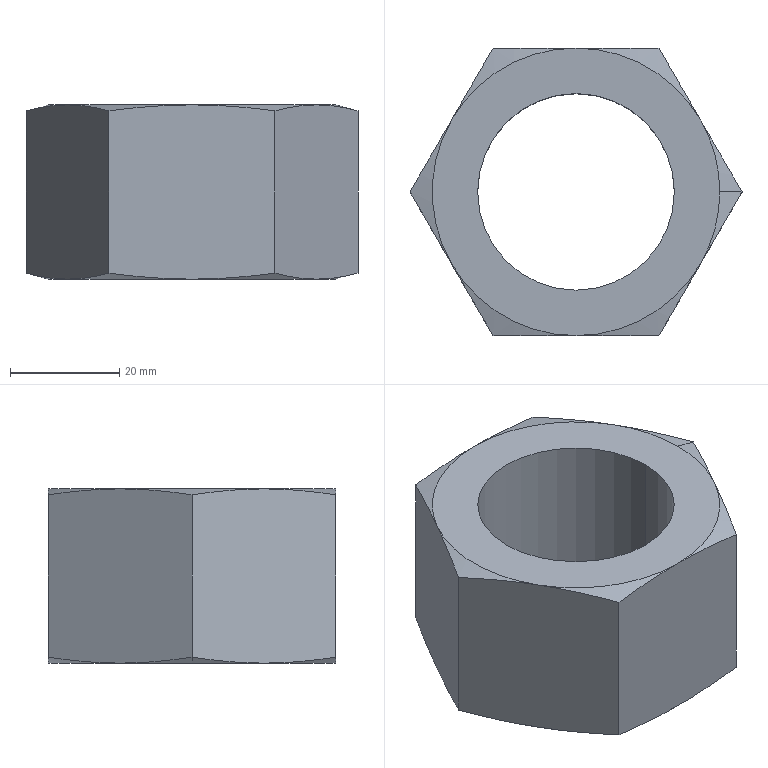Part | SolidWorks | features Cut 2, Chamfer 1, Extrusion 1 | 1 solid | 24 faces | box 60.79 x 52.646 x 31.9 mm | volume 43950 mm3 | cone 14 | plane 8 | cylinder 2 | commonest cylinder face diameters 36 x2
STEP:
#1=CARTESIAN_POINT('',(22.796,13.161,31.9));
#2=VERTEX_POINT('',#1);
#3=CARTESIAN_POINT('',(26.323,0.,31.9));
#4=VERTEX_POINT('',#3);
#5=CARTESIAN_POINT('',(0.,0.,31.9));
#6=DIRECTION('',(0.,0.,-1.));
#7=DIRECTION('',(-1.,0.,0.));
#8=AXIS2_PLACEMENT_3D('',#5,#6,#7);
#9=CIRCLE('',#8,26.323);
#10=EDGE_CURVE('',#2,#4,#9,.T.);
#11=ORIENTED_EDGE('',*,*,#10,.T.);
#12=CARTESIAN_POINT('',(30.395,0.,30.809));
#13=VERTEX_POINT('',#12);
#14=CARTESIAN_POINT('',(26.323,0.,31.9));
#15=DIRECTION('',(0.9659,0.,-0.2588));
#16=VECTOR('',#15,1000.);
#17=LINE('',#14,#16);
#18=EDGE_CURVE('',#4,#13,#17,.T.);
#19=ORIENTED_EDGE('',*,*,#18,.T.);
#20=CARTESIAN_POINT('',(30.395,0.,30.809));
#21=CARTESIAN_POINT('',(29.129,2.194,31.148));
#22=CARTESIAN_POINT('',(27.862,4.387,31.424));
#23=CARTESIAN_POINT('',(25.329,8.774,31.8));
#24=CARTESIAN_POINT('',(24.063,10.968,31.9));
#25=CARTESIAN_POINT('',(22.796,13.161,31.9));
#26=B_SPLINE_CURVE_WITH_KNOTS('',3,(#20,#21,#22,#23,#24,#25),.UNSPECIFIED.,.F.,.F.,(4,2,4),(0.000000231,0.007599,0.0152),.UNSPECIFIED.);
#27=EDGE_CURVE('',#13,#2,#26,.T.);
#28=ORIENTED_EDGE('',*,*,#27,.T.);
#29=EDGE_LOOP('',(#11,#19,#28));
#30=FACE_OUTER_BOUND('',#29,.T.);
#31=CARTESIAN_POINT('',(0.,0.,31.9));
#32=DIRECTION('',(0.,0.,-1.));
#33=DIRECTION('',(1.,0.,0.));
#34=AXIS2_PLACEMENT_3D('',#31,#32,#33);
#35=CONICAL_SURFACE('',#34,26.323,1.309);
#36=ADVANCED_FACE('',(#30),#35,.T.);
#37=CARTESIAN_POINT('',(-26.323,0.,0.));
#38=VERTEX_POINT('',#37);
#39=CARTESIAN_POINT('',(-22.796,13.161,0.));
#40=VERTEX_POINT('',#39);
#41=CARTESIAN_POINT('',(0.,0.,0.));
#42=DIRECTION('',(0.,0.,-1.));
#43=DIRECTION('',(-1.,0.,0.));
#44=AXIS2_PLACEMENT_3D('',#41,#42,#43);
#45=CIRCLE('',#44,26.323);
#46=EDGE_CURVE('',#38,#40,#45,.T.);
#47=ORIENTED_EDGE('',*,*,#46,.F.);
#48=CARTESIAN_POINT('',(-30.395,0.,1.091));
#49=VERTEX_POINT('',#48);
#50=CARTESIAN_POINT('',(-26.323,0.,0.));
#51=DIRECTION('',(-0.9659,0.,0.2588));
#52=VECTOR('',#51,1000.);
#53=LINE('',#50,#52);
#54=EDGE_CURVE('',#38,#49,#53,.T.);
#55=ORIENTED_EDGE('',*,*,#54,.T.);
#56=CARTESIAN_POINT('',(-30.395,0.,1.091));
#57=CARTESIAN_POINT('',(-29.129,2.194,0.7518));
#58=CARTESIAN_POINT('',(-27.862,4.387,0.4762));
#59=CARTESIAN_POINT('',(-25.329,8.774,0.09977));
#60=CARTESIAN_POINT('',(-24.063,10.968,0.));
#61=CARTESIAN_POINT('',(-22.796,13.161,0.));
#62=B_SPLINE_CURVE_WITH_KNOTS('',3,(#56,#57,#58,#59,#60,#61),.UNSPECIFIED.,.F.,.F.,(4,2,4),(0.000000231,0.007599,0.0152),.UNSPECIFIED.);
#63=EDGE_CURVE('',#49,#40,#62,.T.);
#64=ORIENTED_EDGE('',*,*,#63,.T.);
#65=EDGE_LOOP('',(#47,#55,#64));
#66=FACE_OUTER_BOUND('',#65,.T.);
#67=CARTESIAN_POINT('',(0.,0.,0.));
#68=DIRECTION('',(0.,0.,1.));
#69=DIRECTION('',(-1.,0.,0.));
#70=AXIS2_PLACEMENT_3D('',#67,#68,#69);
#71=CONICAL_SURFACE('',#70,26.323,1.309);
#72=ADVANCED_FACE('',(#66),#71,.T.);
#73=CARTESIAN_POINT('',(-18.,0.,31.9));
#74=VERTEX_POINT('',#73);
#75=CARTESIAN_POINT('',(18.,0.,31.9));
#76=VERTEX_POINT('',#75);
#77=CARTESIAN_POINT('',(0.,0.,31.9));
#78=DIRECTION('',(0.,0.,1.));
#79=DIRECTION('',(1.,0.,0.));
#80=AXIS2_PLACEMENT_3D('',#77,#78,#79);
#81=CIRCLE('',#80,18.);
#82=EDGE_CURVE('',#74,#76,#81,.T.);
#83=ORIENTED_EDGE('',*,*,#82,.T.);
#84=CARTESIAN_POINT('',(18.,0.,0.));
#85=VERTEX_POINT('',#84);
#86=CARTESIAN_POINT('',(18.,0.,31.9));
#87=DIRECTION('',(0.,0.,-1.));
#88=VECTOR('',#87,1000.);
#89=LINE('',#86,#88);
#90=EDGE_CURVE('',#76,#85,#89,.T.);
#91=ORIENTED_EDGE('',*,*,#90,.T.);
#92=CARTESIAN_POINT('',(-18.,0.,0.));
#93=VERTEX_POINT('',#92);
#94=CARTESIAN_POINT('',(0.,0.,0.));
#95=DIRECTION('',(0.,0.,1.));
#96=DIRECTION('',(1.,0.,0.));
#97=AXIS2_PLACEMENT_3D('',#94,#95,#96);
#98=CIRCLE('',#97,18.);
#99=EDGE_CURVE('',#93,#85,#98,.T.);
#100=ORIENTED_EDGE('',*,*,#99,.F.);
#101=CARTESIAN_POINT('',(-18.,0.,31.9));
#102=DIRECTION('',(0.,0.,-1.));
#103=VECTOR('',#102,1000.);
#104=LINE('',#101,#103);
#105=EDGE_CURVE('',#74,#93,#104,.T.);
#106=ORIENTED_EDGE('',*,*,#105,.F.);
#107=EDGE_LOOP('',(#83,#91,#100,#106));
#108=FACE_OUTER_BOUND('',#107,.T.);
#109=CARTESIAN_POINT('',(0.,0.,31.9));
#110=DIRECTION('',(0.,0.,-1.));
#111=DIRECTION('',(-1.,0.,0.));
#112=AXIS2_PLACEMENT_3D('',#109,#110,#111);
#113=CYLINDRICAL_SURFACE('',#112,18.);
#114=ADVANCED_FACE('',(#108),#113,.F.);
#115=ORIENTED_EDGE('',*,*,#27,.F.);
#116=CARTESIAN_POINT('',(30.395,0.,1.091));
#117=VERTEX_POINT('',#116);
#118=CARTESIAN_POINT('',(30.395,0.,31.9));
#119=DIRECTION('',(0.,0.,-1.));
#120=VECTOR('',#119,1000.);
#121=LINE('',#118,#120);
#122=EDGE_CURVE('',#13,#117,#121,.T.);
#123=ORIENTED_EDGE('',*,*,#122,.T.);
#124=CARTESIAN_POINT('',(22.796,13.161,0.));
#125=VERTEX_POINT('',#124);
#126=CARTESIAN_POINT('',(22.796,13.161,0.));
#127=CARTESIAN_POINT('',(24.063,10.968,0.));
#128=CARTESIAN_POINT('',(25.329,8.774,0.09977));
#129=CARTESIAN_POINT('',(27.862,4.387,0.4762));
#130=CARTESIAN_POINT('',(29.129,2.194,0.7518));
#131=CARTESIAN_POINT('',(30.395,0.,1.091));
#132=B_SPLINE_CURVE_WITH_KNOTS('',3,(#126,#127,#128,#129,#130,#131),.UNSPECIFIED.,.F.,.F.,(4,2,4),(0.0152,0.0228,0.0304),.UNSPECIFIED.);
#133=EDGE_CURVE('',#125,#117,#132,.T.);
#134=ORIENTED_EDGE('',*,*,#133,.F.);
#135=CARTESIAN_POINT('',(15.198,26.323,1.091));
#136=VERTEX_POINT('',#135);
#137=CARTESIAN_POINT('',(15.198,26.323,1.091));
#138=CARTESIAN_POINT('',(16.464,24.129,0.7518));
#139=CARTESIAN_POINT('',(17.73,21.936,0.4762));
#140=CARTESIAN_POINT('',(20.263,17.549,0.09977));
#141=CARTESIAN_POINT('',(21.53,15.355,0.));
#142=CARTESIAN_POINT('',(22.796,13.161,0.));
#143=B_SPLINE_CURVE_WITH_KNOTS('',3,(#137,#138,#139,#140,#141,#142),.UNSPECIFIED.,.F.,.F.,(4,2,4),(0.000000231,0.007599,0.0152),.UNSPECIFIED.);
#144=EDGE_CURVE('',#136,#125,#143,.T.);
#145=ORIENTED_EDGE('',*,*,#144,.F.);
#146=CARTESIAN_POINT('',(15.198,26.323,30.809));
#147=VERTEX_POINT('',#146);
#148=CARTESIAN_POINT('',(15.198,26.323,31.9));
#149=DIRECTION('',(0.,0.,-1.));
#150=VECTOR('',#149,1000.);
#151=LINE('',#148,#150);
#152=EDGE_CURVE('',#147,#136,#151,.T.);
#153=ORIENTED_EDGE('',*,*,#152,.F.);
#154=CARTESIAN_POINT('',(22.796,13.161,31.9));
#155=CARTESIAN_POINT('',(21.53,15.355,31.9));
#156=CARTESIAN_POINT('',(20.263,17.549,31.8));
#157=CARTESIAN_POINT('',(17.73,21.936,31.424));
#158=CARTESIAN_POINT('',(16.464,24.129,31.148));
#159=CARTESIAN_POINT('',(15.198,26.323,30.809));
#160=B_SPLINE_CURVE_WITH_KNOTS('',3,(#154,#155,#156,#157,#158,#159),.UNSPECIFIED.,.F.,.F.,(4,2,4),(0.0152,0.0228,0.0304),.UNSPECIFIED.);
#161=EDGE_CURVE('',#2,#147,#160,.T.);
#162=ORIENTED_EDGE('',*,*,#161,.F.);
#163=EDGE_LOOP('',(#115,#123,#134,#145,#153,#162));
#164=FACE_OUTER_BOUND('',#163,.T.);
#165=CARTESIAN_POINT('',(30.395,0.,31.9));
#166=DIRECTION('',(-0.866,-0.5,0.));
#167=DIRECTION('',(0.5,-0.866,0.));
#168=AXIS2_PLACEMENT_3D('',#165,#166,#167);
#169=PLANE('',#168);
#170=ADVANCED_FACE('',(#164),#169,.F.);
#171=CARTESIAN_POINT('',(0.,26.323,31.9));
#172=VERTEX_POINT('',#171);
#173=CARTESIAN_POINT('',(15.198,26.323,30.809));
#174=CARTESIAN_POINT('',(12.669,26.323,31.148));
#175=CARTESIAN_POINT('',(10.138,26.323,31.423));
#176=CARTESIAN_POINT('',(5.073,26.323,31.8));
#177=CARTESIAN_POINT('',(2.538,26.323,31.9));
#178=CARTESIAN_POINT('',(0.,26.323,31.9));
#179=B_SPLINE_CURVE_WITH_KNOTS('',3,(#173,#174,#175,#176,#177,#178),.UNSPECIFIED.,.F.,.F.,(4,2,4),(0.08306,0.0907,0.09835),.UNSPECIFIED.);
#180=EDGE_CURVE('',#147,#172,#179,.T.);
#181=ORIENTED_EDGE('',*,*,#180,.F.);
#182=ORIENTED_EDGE('',*,*,#152,.T.);
#183=CARTESIAN_POINT('',(0.,26.323,0.));
#184=VERTEX_POINT('',#183);
#185=CARTESIAN_POINT('',(0.,26.323,0.));
#186=CARTESIAN_POINT('',(2.538,26.323,0.));
#187=CARTESIAN_POINT('',(5.073,26.323,0.1001));
#188=CARTESIAN_POINT('',(10.138,26.323,0.4769));
#189=CARTESIAN_POINT('',(12.669,26.323,0.7524));
#190=CARTESIAN_POINT('',(15.198,26.323,1.091));
#191=B_SPLINE_CURVE_WITH_KNOTS('',3,(#185,#186,#187,#188,#189,#190),.UNSPECIFIED.,.F.,.F.,(4,2,4),(0.04121,0.04887,0.05653),.UNSPECIFIED.);
#192=EDGE_CURVE('',#184,#136,#191,.T.);
#193=ORIENTED_EDGE('',*,*,#192,.F.);
#194=CARTESIAN_POINT('',(-15.197,26.323,1.091));
#195=VERTEX_POINT('',#194);
#196=CARTESIAN_POINT('',(-15.197,26.323,1.091));
#197=CARTESIAN_POINT('',(-12.672,26.323,0.7527));
#198=CARTESIAN_POINT('',(-10.131,26.323,0.4761));
#199=CARTESIAN_POINT('',(-5.062,26.323,0.09952));
#200=CARTESIAN_POINT('',(-2.53,26.323,0.));
#201=CARTESIAN_POINT('',(0.,26.323,0.));
#202=B_SPLINE_CURVE_WITH_KNOTS('',3,(#196,#197,#198,#199,#200,#201),.UNSPECIFIED.,.F.,.F.,(4,2,4),(0.02593,0.03357,0.04121),.UNSPECIFIED.);
#203=EDGE_CURVE('',#195,#184,#202,.T.);
#204=ORIENTED_EDGE('',*,*,#203,.F.);
#205=CARTESIAN_POINT('',(-15.197,26.323,30.809));
#206=VERTEX_POINT('',#205);
#207=CARTESIAN_POINT('',(-15.197,26.323,31.9));
#208=DIRECTION('',(0.,0.,-1.));
#209=VECTOR('',#208,1000.);
#210=LINE('',#207,#209);
#211=EDGE_CURVE('',#206,#195,#210,.T.);
#212=ORIENTED_EDGE('',*,*,#211,.F.);
#213=CARTESIAN_POINT('',(0.,26.323,31.9));
#214=CARTESIAN_POINT('',(-2.53,26.323,31.9));
#215=CARTESIAN_POINT('',(-5.062,26.323,31.8));
#216=CARTESIAN_POINT('',(-10.131,26.323,31.424));
#217=CARTESIAN_POINT('',(-12.672,26.323,31.147));
#218=CARTESIAN_POINT('',(-15.197,26.323,30.809));
#219=B_SPLINE_CURVE_WITH_KNOTS('',3,(#213,#214,#215,#216,#217,#218),.UNSPECIFIED.,.F.,.F.,(4,2,4),(0.09835,0.106,0.1136),.UNSPECIFIED.);
#220=EDGE_CURVE('',#172,#206,#219,.T.);
#221=ORIENTED_EDGE('',*,*,#220,.F.);
#222=EDGE_LOOP('',(#181,#182,#193,#204,#212,#221));
#223=FACE_OUTER_BOUND('',#222,.T.);
#224=CARTESIAN_POINT('',(15.198,26.323,31.9));
#225=DIRECTION('',(0.,-1.,0.));
#226=DIRECTION('',(1.,0.,0.));
#227=AXIS2_PLACEMENT_3D('',#224,#225,#226);
#228=PLANE('',#227);
#229=ADVANCED_FACE('',(#223),#228,.F.);
#230=CARTESIAN_POINT('',(-22.796,13.161,31.9));
#231=VERTEX_POINT('',#230);
#232=CARTESIAN_POINT('',(-15.197,26.323,30.809));
#233=CARTESIAN_POINT('',(-16.464,24.129,31.148));
#234=CARTESIAN_POINT('',(-17.73,21.936,31.424));
#235=CARTESIAN_POINT('',(-20.263,17.549,31.8));
#236=CARTESIAN_POINT('',(-21.53,15.355,31.9));
#237=CARTESIAN_POINT('',(-22.796,13.161,31.9));
#238=B_SPLINE_CURVE_WITH_KNOTS('',3,(#232,#233,#234,#235,#236,#237),.UNSPECIFIED.,.F.,.F.,(4,2,4),(0.000000231,0.007599,0.0152),.UNSPECIFIED.);
#239=EDGE_CURVE('',#206,#231,#238,.T.);
#240=ORIENTED_EDGE('',*,*,#239,.F.);
#241=ORIENTED_EDGE('',*,*,#211,.T.);
#242=CARTESIAN_POINT('',(-22.796,13.161,0.));
#243=CARTESIAN_POINT('',(-21.53,15.355,0.));
#244=CARTESIAN_POINT('',(-20.263,17.549,0.09977));
#245=CARTESIAN_POINT('',(-17.73,21.936,0.4762));
#246=CARTESIAN_POINT('',(-16.464,24.129,0.7518));
#247=CARTESIAN_POINT('',(-15.197,26.323,1.091));
#248=B_SPLINE_CURVE_WITH_KNOTS('',3,(#242,#243,#244,#245,#246,#247),.UNSPECIFIED.,.F.,.F.,(4,2,4),(0.0152,0.0228,0.0304),.UNSPECIFIED.);
#249=EDGE_CURVE('',#40,#195,#248,.T.);
#250=ORIENTED_EDGE('',*,*,#249,.F.);
#251=ORIENTED_EDGE('',*,*,#63,.F.);
#252=CARTESIAN_POINT('',(-30.395,0.,30.809));
#253=VERTEX_POINT('',#252);
#254=CARTESIAN_POINT('',(-30.395,0.,31.9));
#255=DIRECTION('',(0.,0.,-1.));
#256=VECTOR('',#255,1000.);
#257=LINE('',#254,#256);
#258=EDGE_CURVE('',#253,#49,#257,.T.);
#259=ORIENTED_EDGE('',*,*,#258,.F.);
#260=CARTESIAN_POINT('',(-22.796,13.161,31.9));
#261=CARTESIAN_POINT('',(-24.063,10.968,31.9));
#262=CARTESIAN_POINT('',(-25.329,8.774,31.8));
#263=CARTESIAN_POINT('',(-27.862,4.387,31.424));
#264=CARTESIAN_POINT('',(-29.129,2.194,31.148));
#265=CARTESIAN_POINT('',(-30.395,0.,30.809));
#266=B_SPLINE_CURVE_WITH_KNOTS('',3,(#260,#261,#262,#263,#264,#265),.UNSPECIFIED.,.F.,.F.,(4,2,4),(0.0152,0.0228,0.0304),.UNSPECIFIED.);
#267=EDGE_CURVE('',#231,#253,#266,.T.);
#268=ORIENTED_EDGE('',*,*,#267,.F.);
#269=EDGE_LOOP('',(#240,#241,#250,#251,#259,#268));
#270=FACE_OUTER_BOUND('',#269,.T.);
#271=CARTESIAN_POINT('',(-15.197,26.323,31.9));
#272=DIRECTION('',(0.866,-0.5,0.));
#273=DIRECTION('',(0.5,0.866,0.));
#274=AXIS2_PLACEMENT_3D('',#271,#272,#273);
#275=PLANE('',#274);
#276=ADVANCED_FACE('',(#270),#275,.F.);
#277=CARTESIAN_POINT('',(-22.796,-13.161,31.9));
#278=VERTEX_POINT('',#277);
#279=CARTESIAN_POINT('',(-30.395,0.,30.809));
#280=CARTESIAN_POINT('',(-29.129,-2.194,31.148));
#281=CARTESIAN_POINT('',(-27.862,-4.387,31.424));
#282=CARTESIAN_POINT('',(-25.329,-8.774,31.8));
#283=CARTESIAN_POINT('',(-24.063,-10.968,31.9));
#284=CARTESIAN_POINT('',(-22.796,-13.161,31.9));
#285=B_SPLINE_CURVE_WITH_KNOTS('',3,(#279,#280,#281,#282,#283,#284),.UNSPECIFIED.,.F.,.F.,(4,2,4),(0.000000231,0.007599,0.0152),.UNSPECIFIED.);
#286=EDGE_CURVE('',#253,#278,#285,.T.);
#287=ORIENTED_EDGE('',*,*,#286,.F.);
#288=ORIENTED_EDGE('',*,*,#258,.T.);
#289=CARTESIAN_POINT('',(-22.796,-13.161,0.));
#290=VERTEX_POINT('',#289);
#291=CARTESIAN_POINT('',(-22.796,-13.161,0.));
#292=CARTESIAN_POINT('',(-24.063,-10.968,0.));
#293=CARTESIAN_POINT('',(-25.329,-8.774,0.09977));
#294=CARTESIAN_POINT('',(-27.862,-4.387,0.4762));
#295=CARTESIAN_POINT('',(-29.129,-2.194,0.7518));
#296=CARTESIAN_POINT('',(-30.395,0.,1.091));
#297=B_SPLINE_CURVE_WITH_KNOTS('',3,(#291,#292,#293,#294,#295,#296),.UNSPECIFIED.,.F.,.F.,(4,2,4),(0.0152,0.0228,0.0304),.UNSPECIFIED.);
#298=EDGE_CURVE('',#290,#49,#297,.T.);
#299=ORIENTED_EDGE('',*,*,#298,.F.);
#300=CARTESIAN_POINT('',(-15.198,-26.323,1.091));
#301=VERTEX_POINT('',#300);
#302=CARTESIAN_POINT('',(-15.198,-26.323,1.091));
#303=CARTESIAN_POINT('',(-16.464,-24.129,0.7518));
#304=CARTESIAN_POINT('',(-17.73,-21.936,0.4762));
#305=CARTESIAN_POINT('',(-20.263,-17.549,0.09977));
#306=CARTESIAN_POINT('',(-21.53,-15.355,0.));
#307=CARTESIAN_POINT('',(-22.796,-13.161,0.));
#308=B_SPLINE_CURVE_WITH_KNOTS('',3,(#302,#303,#304,#305,#306,#307),.UNSPECIFIED.,.F.,.F.,(4,2,4),(0.000000231,0.007599,0.0152),.UNSPECIFIED.);
#309=EDGE_CURVE('',#301,#290,#308,.T.);
#310=ORIENTED_EDGE('',*,*,#309,.F.);
#311=CARTESIAN_POINT('',(-15.198,-26.323,30.809));
#312=VERTEX_POINT('',#311);
#313=CARTESIAN_POINT('',(-15.197,-26.323,31.9));
#314=DIRECTION('',(0.,0.,-1.));
#315=VECTOR('',#314,1000.);
#316=LINE('',#313,#315);
#317=EDGE_CURVE('',#312,#301,#316,.T.);
#318=ORIENTED_EDGE('',*,*,#317,.F.);
#319=CARTESIAN_POINT('',(-22.796,-13.161,31.9));
#320=CARTESIAN_POINT('',(-21.53,-15.355,31.9));
#321=CARTESIAN_POINT('',(-20.263,-17.549,31.8));
#322=CARTESIAN_POINT('',(-17.73,-21.936,31.424));
#323=CARTESIAN_POINT('',(-16.464,-24.129,31.148));
#324=CARTESIAN_POINT('',(-15.198,-26.323,30.809));
#325=B_SPLINE_CURVE_WITH_KNOTS('',3,(#319,#320,#321,#322,#323,#324),.UNSPECIFIED.,.F.,.F.,(4,2,4),(0.0152,0.0228,0.0304),.UNSPECIFIED.);
#326=EDGE_CURVE('',#278,#312,#325,.T.);
#327=ORIENTED_EDGE('',*,*,#326,.F.);
#328=EDGE_LOOP('',(#287,#288,#299,#310,#318,#327));
#329=FACE_OUTER_BOUND('',#328,.T.);
#330=CARTESIAN_POINT('',(-30.395,0.,31.9));
#331=DIRECTION('',(0.866,0.5,0.));
#332=DIRECTION('',(-0.5,0.866,0.));
#333=AXIS2_PLACEMENT_3D('',#330,#331,#332);
#334=PLANE('',#333);
#335=ADVANCED_FACE('',(#329),#334,.F.);
#336=CARTESIAN_POINT('',(0.,-26.323,31.9));
#337=VERTEX_POINT('',#336);
#338=CARTESIAN_POINT('',(-15.198,-26.323,30.809));
#339=CARTESIAN_POINT('',(-12.672,-26.323,31.147));
#340=CARTESIAN_POINT('',(-10.131,-26.323,31.424));
#341=CARTESIAN_POINT('',(-5.062,-26.323,31.8));
#342=CARTESIAN_POINT('',(-2.53,-26.323,31.9));
#343=CARTESIAN_POINT('',(0.,-26.323,31.9));
#344=B_SPLINE_CURVE_WITH_KNOTS('',3,(#338,#339,#340,#341,#342,#343),.UNSPECIFIED.,.F.,.F.,(4,2,4),(0.02593,0.03357,0.04121),.UNSPECIFIED.);
#345=EDGE_CURVE('',#312,#337,#344,.T.);
#346=ORIENTED_EDGE('',*,*,#345,.F.);
#347=ORIENTED_EDGE('',*,*,#317,.T.);
#348=CARTESIAN_POINT('',(0.,-26.323,0.));
#349=VERTEX_POINT('',#348);
#350=CARTESIAN_POINT('',(0.,-26.323,0.));
#351=CARTESIAN_POINT('',(-2.53,-26.323,0.));
#352=CARTESIAN_POINT('',(-5.062,-26.323,0.09952));
#353=CARTESIAN_POINT('',(-10.131,-26.323,0.4761));
#354=CARTESIAN_POINT('',(-12.672,-26.323,0.7527));
#355=CARTESIAN_POINT('',(-15.198,-26.323,1.091));
#356=B_SPLINE_CURVE_WITH_KNOTS('',3,(#350,#351,#352,#353,#354,#355),.UNSPECIFIED.,.F.,.F.,(4,2,4),(0.09835,0.106,0.1136),.UNSPECIFIED.);
#357=EDGE_CURVE('',#349,#301,#356,.T.);
#358=ORIENTED_EDGE('',*,*,#357,.F.);
#359=CARTESIAN_POINT('',(15.198,-26.323,1.091));
#360=VERTEX_POINT('',#359);
#361=CARTESIAN_POINT('',(15.198,-26.323,1.091));
#362=CARTESIAN_POINT('',(12.669,-26.323,0.7524));
#363=CARTESIAN_POINT('',(10.138,-26.323,0.4769));
#364=CARTESIAN_POINT('',(5.073,-26.323,0.1001));
#365=CARTESIAN_POINT('',(2.538,-26.323,0.));
#366=CARTESIAN_POINT('',(0.,-26.323,0.));
#367=B_SPLINE_CURVE_WITH_KNOTS('',3,(#361,#362,#363,#364,#365,#366),.UNSPECIFIED.,.F.,.F.,(4,2,4),(0.08306,0.0907,0.09835),.UNSPECIFIED.);
#368=EDGE_CURVE('',#360,#349,#367,.T.);
#369=ORIENTED_EDGE('',*,*,#368,.F.);
#370=CARTESIAN_POINT('',(15.198,-26.323,30.809));
#371=VERTEX_POINT('',#370);
#372=CARTESIAN_POINT('',(15.198,-26.323,31.9));
#373=DIRECTION('',(0.,0.,-1.));
#374=VECTOR('',#373,1000.);
#375=LINE('',#372,#374);
#376=EDGE_CURVE('',#371,#360,#375,.T.);
#377=ORIENTED_EDGE('',*,*,#376,.F.);
#378=CARTESIAN_POINT('',(0.,-26.323,31.9));
#379=CARTESIAN_POINT('',(2.538,-26.323,31.9));
#380=CARTESIAN_POINT('',(5.073,-26.323,31.8));
#381=CARTESIAN_POINT('',(10.138,-26.323,31.423));
#382=CARTESIAN_POINT('',(12.669,-26.323,31.148));
#383=CARTESIAN_POINT('',(15.198,-26.323,30.809));
#384=B_SPLINE_CURVE_WITH_KNOTS('',3,(#378,#379,#380,#381,#382,#383),.UNSPECIFIED.,.F.,.F.,(4,2,4),(0.04121,0.04887,0.05653),.UNSPECIFIED.);
#385=EDGE_CURVE('',#337,#371,#384,.T.);
#386=ORIENTED_EDGE('',*,*,#385,.F.);
#387=EDGE_LOOP('',(#346,#347,#358,#369,#377,#386));
#388=FACE_OUTER_BOUND('',#387,.T.);
#389=CARTESIAN_POINT('',(-15.197,-26.323,31.9));
#390=DIRECTION('',(0.,1.,0.));
#391=DIRECTION('',(-1.,0.,0.));
#392=AXIS2_PLACEMENT_3D('',#389,#390,#391);
#393=PLANE('',#392);
#394=ADVANCED_FACE('',(#388),#393,.F.);
#395=CARTESIAN_POINT('',(22.796,-13.161,31.9));
#396=VERTEX_POINT('',#395);
#397=CARTESIAN_POINT('',(15.198,-26.323,30.809));
#398=CARTESIAN_POINT('',(16.464,-24.129,31.148));
#399=CARTESIAN_POINT('',(17.73,-21.936,31.424));
#400=CARTESIAN_POINT('',(20.263,-17.549,31.8));
#401=CARTESIAN_POINT('',(21.53,-15.355,31.9));
#402=CARTESIAN_POINT('',(22.796,-13.161,31.9));
#403=B_SPLINE_CURVE_WITH_KNOTS('',3,(#397,#398,#399,#400,#401,#402),.UNSPECIFIED.,.F.,.F.,(4,2,4),(0.000000231,0.007599,0.0152),.UNSPECIFIED.);
#404=EDGE_CURVE('',#371,#396,#403,.T.);
#405=ORIENTED_EDGE('',*,*,#404,.F.);
#406=ORIENTED_EDGE('',*,*,#376,.T.);
#407=CARTESIAN_POINT('',(22.796,-13.161,0.));
#408=VERTEX_POINT('',#407);
#409=CARTESIAN_POINT('',(22.796,-13.161,0.));
#410=CARTESIAN_POINT('',(21.53,-15.355,0.));
#411=CARTESIAN_POINT('',(20.263,-17.549,0.09977));
#412=CARTESIAN_POINT('',(17.73,-21.936,0.4762));
#413=CARTESIAN_POINT('',(16.464,-24.129,0.7518));
#414=CARTESIAN_POINT('',(15.198,-26.323,1.091));
#415=B_SPLINE_CURVE_WITH_KNOTS('',3,(#409,#410,#411,#412,#413,#414),.UNSPECIFIED.,.F.,.F.,(4,2,4),(0.0152,0.0228,0.0304),.UNSPECIFIED.);
#416=EDGE_CURVE('',#408,#360,#415,.T.);
#417=ORIENTED_EDGE('',*,*,#416,.F.);
#418=CARTESIAN_POINT('',(30.395,0.,1.091));
#419=CARTESIAN_POINT('',(29.129,-2.194,0.7518));
#420=CARTESIAN_POINT('',(27.862,-4.387,0.4762));
#421=CARTESIAN_POINT('',(25.329,-8.774,0.09977));
#422=CARTESIAN_POINT('',(24.063,-10.968,0.));
#423=CARTESIAN_POINT('',(22.796,-13.161,0.));
#424=B_SPLINE_CURVE_WITH_KNOTS('',3,(#418,#419,#420,#421,#422,#423),.UNSPECIFIED.,.F.,.F.,(4,2,4),(0.000000231,0.007599,0.0152),.UNSPECIFIED.);
#425=EDGE_CURVE('',#117,#408,#424,.T.);
#426=ORIENTED_EDGE('',*,*,#425,.F.);
#427=ORIENTED_EDGE('',*,*,#122,.F.);
#428=CARTESIAN_POINT('',(22.796,-13.161,31.9));
#429=CARTESIAN_POINT('',(24.063,-10.968,31.9));
#430=CARTESIAN_POINT('',(25.329,-8.774,31.8));
#431=CARTESIAN_POINT('',(27.862,-4.387,31.424));
#432=CARTESIAN_POINT('',(29.129,-2.194,31.148));
#433=CARTESIAN_POINT('',(30.395,0.,30.809));
#434=B_SPLINE_CURVE_WITH_KNOTS('',3,(#428,#429,#430,#431,#432,#433),.UNSPECIFIED.,.F.,.F.,(4,2,4),(0.0152,0.0228,0.0304),.UNSPECIFIED.);
#435=EDGE_CURVE('',#396,#13,#434,.T.);
#436=ORIENTED_EDGE('',*,*,#435,.F.);
#437=EDGE_LOOP('',(#405,#406,#417,#426,#427,#436));
#438=FACE_OUTER_BOUND('',#437,.T.);
#439=CARTESIAN_POINT('',(15.198,-26.323,31.9));
#440=DIRECTION('',(-0.866,0.5,0.));
#441=DIRECTION('',(-0.5,-0.866,0.));
#442=AXIS2_PLACEMENT_3D('',#439,#440,#441);
#443=PLANE('',#442);
#444=ADVANCED_FACE('',(#438),#443,.F.);
#445=ORIENTED_EDGE('',*,*,#82,.F.);
#446=CARTESIAN_POINT('',(0.,0.,31.9));
#447=DIRECTION('',(0.,0.,1.));
#448=DIRECTION('',(1.,0.,0.));
#449=AXIS2_PLACEMENT_3D('',#446,#447,#448);
#450=CIRCLE('',#449,18.);
#451=EDGE_CURVE('',#76,#74,#450,.T.);
#452=ORIENTED_EDGE('',*,*,#451,.F.);
#453=EDGE_LOOP('',(#445,#452));
#454=FACE_BOUND('',#453,.T.);
#455=CARTESIAN_POINT('',(0.,0.,31.9));
#456=DIRECTION('',(0.,0.,-1.));
#457=DIRECTION('',(-1.,0.,0.));
#458=AXIS2_PLACEMENT_3D('',#455,#456,#457);
#459=CIRCLE('',#458,26.323);
#460=EDGE_CURVE('',#231,#172,#459,.T.);
#461=ORIENTED_EDGE('',*,*,#460,.F.);
#462=CARTESIAN_POINT('',(0.,0.,31.9));
#463=DIRECTION('',(0.,0.,-1.));
#464=DIRECTION('',(-1.,0.,0.));
#465=AXIS2_PLACEMENT_3D('',#462,#463,#464);
#466=CIRCLE('',#465,26.323);
#467=EDGE_CURVE('',#278,#231,#466,.T.);
#468=ORIENTED_EDGE('',*,*,#467,.F.);
#469=CARTESIAN_POINT('',(0.,0.,31.9));
#470=DIRECTION('',(0.,0.,-1.));
#471=DIRECTION('',(-1.,0.,0.));
#472=AXIS2_PLACEMENT_3D('',#469,#470,#471);
#473=CIRCLE('',#472,26.323);
#474=EDGE_CURVE('',#337,#278,#473,.T.);
#475=ORIENTED_EDGE('',*,*,#474,.F.);
#476=CARTESIAN_POINT('',(0.,0.,31.9));
#477=DIRECTION('',(0.,0.,-1.));
#478=DIRECTION('',(-1.,0.,0.));
#479=AXIS2_PLACEMENT_3D('',#476,#477,#478);
#480=CIRCLE('',#479,26.323);
#481=EDGE_CURVE('',#396,#337,#480,.T.);
#482=ORIENTED_EDGE('',*,*,#481,.F.);
#483=CARTESIAN_POINT('',(0.,0.,31.9));
#484=DIRECTION('',(0.,0.,-1.));
#485=DIRECTION('',(-1.,0.,0.));
#486=AXIS2_PLACEMENT_3D('',#483,#484,#485);
#487=CIRCLE('',#486,26.323);
#488=EDGE_CURVE('',#4,#396,#487,.T.);
#489=ORIENTED_EDGE('',*,*,#488,.F.);
#490=ORIENTED_EDGE('',*,*,#10,.F.);
#491=CARTESIAN_POINT('',(0.,0.,31.9));
#492=DIRECTION('',(0.,0.,1.));
#493=DIRECTION('',(1.,0.,0.));
#494=AXIS2_PLACEMENT_3D('',#491,#492,#493);
#495=CIRCLE('',#494,26.323);
#496=EDGE_CURVE('',#2,#172,#495,.T.);
#497=ORIENTED_EDGE('',*,*,#496,.T.);
#498=EDGE_LOOP('',(#461,#468,#475,#482,#489,#490,#497));
#499=FACE_OUTER_BOUND('',#498,.T.);
#500=CARTESIAN_POINT('',(45.592,-26.323,31.9));
#501=DIRECTION('',(0.,0.,-1.));
#502=DIRECTION('',(-1.,0.,0.));
#503=AXIS2_PLACEMENT_3D('',#500,#501,#502);
#504=PLANE('',#503);
#505=ADVANCED_FACE('',(#454,#499),#504,.F.);
#506=ORIENTED_EDGE('',*,*,#99,.T.);
#507=CARTESIAN_POINT('',(0.,0.,0.));
#508=DIRECTION('',(0.,0.,1.));
#509=DIRECTION('',(1.,0.,0.));
#510=AXIS2_PLACEMENT_3D('',#507,#508,#509);
#511=CIRCLE('',#510,18.);
#512=EDGE_CURVE('',#85,#93,#511,.T.);
#513=ORIENTED_EDGE('',*,*,#512,.T.);
#514=EDGE_LOOP('',(#506,#513));
#515=FACE_BOUND('',#514,.T.);
#516=CARTESIAN_POINT('',(0.,0.,0.));
#517=DIRECTION('',(0.,0.,-1.));
#518=DIRECTION('',(-1.,0.,0.));
#519=AXIS2_PLACEMENT_3D('',#516,#517,#518);
#520=CIRCLE('',#519,26.323);
#521=EDGE_CURVE('',#290,#38,#520,.T.);
#522=ORIENTED_EDGE('',*,*,#521,.T.);
#523=ORIENTED_EDGE('',*,*,#46,.T.);
#524=CARTESIAN_POINT('',(0.,0.,0.));
#525=DIRECTION('',(0.,0.,-1.));
#526=DIRECTION('',(-1.,0.,0.));
#527=AXIS2_PLACEMENT_3D('',#524,#525,#526);
#528=CIRCLE('',#527,26.323);
#529=EDGE_CURVE('',#40,#184,#528,.T.);
#530=ORIENTED_EDGE('',*,*,#529,.T.);
#531=CARTESIAN_POINT('',(0.,0.,0.));
#532=DIRECTION('',(0.,0.,-1.));
#533=DIRECTION('',(-1.,0.,0.));
#534=AXIS2_PLACEMENT_3D('',#531,#532,#533);
#535=CIRCLE('',#534,26.323);
#536=EDGE_CURVE('',#184,#125,#535,.T.);
#537=ORIENTED_EDGE('',*,*,#536,.T.);
#538=CARTESIAN_POINT('',(0.,0.,0.));
#539=DIRECTION('',(0.,0.,-1.));
#540=DIRECTION('',(-1.,0.,0.));
#541=AXIS2_PLACEMENT_3D('',#538,#539,#540);
#542=CIRCLE('',#541,26.323);
#543=EDGE_CURVE('',#125,#408,#542,.T.);
#544=ORIENTED_EDGE('',*,*,#543,.T.);
#545=CARTESIAN_POINT('',(0.,0.,0.));
#546=DIRECTION('',(0.,0.,-1.));
#547=DIRECTION('',(-1.,0.,0.));
#548=AXIS2_PLACEMENT_3D('',#545,#546,#547);
#549=CIRCLE('',#548,26.323);
#550=EDGE_CURVE('',#408,#349,#549,.T.);
#551=ORIENTED_EDGE('',*,*,#550,.T.);
#552=CARTESIAN_POINT('',(0.,0.,0.));
#553=DIRECTION('',(0.,0.,-1.));
#554=DIRECTION('',(-1.,0.,0.));
#555=AXIS2_PLACEMENT_3D('',#552,#553,#554);
#556=CIRCLE('',#555,26.323);
#557=EDGE_CURVE('',#349,#290,#556,.T.);
#558=ORIENTED_EDGE('',*,*,#557,.T.);
#559=EDGE_LOOP('',(#522,#523,#530,#537,#544,#551,#558));
#560=FACE_OUTER_BOUND('',#559,.T.);
#561=CARTESIAN_POINT('',(45.592,-26.323,0.));
#562=DIRECTION('',(0.,0.,-1.));
#563=DIRECTION('',(-1.,0.,0.));
#564=AXIS2_PLACEMENT_3D('',#561,#562,#563);
#565=PLANE('',#564);
#566=ADVANCED_FACE('',(#515,#560),#565,.T.);
#567=ORIENTED_EDGE('',*,*,#90,.F.);
#568=ORIENTED_EDGE('',*,*,#451,.T.);
#569=ORIENTED_EDGE('',*,*,#105,.T.);
#570=ORIENTED_EDGE('',*,*,#512,.F.);
#571=EDGE_LOOP('',(#567,#568,#569,#570));
#572=FACE_OUTER_BOUND('',#571,.T.);
#573=CARTESIAN_POINT('',(0.,0.,31.9));
#574=DIRECTION('',(0.,0.,-1.));
#575=DIRECTION('',(-1.,0.,0.));
#576=AXIS2_PLACEMENT_3D('',#573,#574,#575);
#577=CYLINDRICAL_SURFACE('',#576,18.);
#578=ADVANCED_FACE('',(#572),#577,.F.);
#579=ORIENTED_EDGE('',*,*,#368,.T.);
#580=ORIENTED_EDGE('',*,*,#550,.F.);
#581=ORIENTED_EDGE('',*,*,#416,.T.);
#582=EDGE_LOOP('',(#579,#580,#581));
#583=FACE_OUTER_BOUND('',#582,.T.);
#584=CARTESIAN_POINT('',(0.,0.,0.));
#585=DIRECTION('',(0.,0.,1.));
#586=DIRECTION('',(-1.,0.,0.));
#587=AXIS2_PLACEMENT_3D('',#584,#585,#586);
#588=CONICAL_SURFACE('',#587,26.323,1.309);
#589=ADVANCED_FACE('',(#583),#588,.T.);
#590=ORIENTED_EDGE('',*,*,#133,.T.);
#591=ORIENTED_EDGE('',*,*,#425,.T.);
#592=ORIENTED_EDGE('',*,*,#543,.F.);
#593=EDGE_LOOP('',(#590,#591,#592));
#594=FACE_OUTER_BOUND('',#593,.T.);
#595=CARTESIAN_POINT('',(0.,0.,0.));
#596=DIRECTION('',(0.,0.,1.));
#597=DIRECTION('',(-1.,0.,0.));
#598=AXIS2_PLACEMENT_3D('',#595,#596,#597);
#599=CONICAL_SURFACE('',#598,26.323,1.309);
#600=ADVANCED_FACE('',(#594),#599,.T.);
#601=ORIENTED_EDGE('',*,*,#309,.T.);
#602=ORIENTED_EDGE('',*,*,#557,.F.);
#603=ORIENTED_EDGE('',*,*,#357,.T.);
#604=EDGE_LOOP('',(#601,#602,#603));
#605=FACE_OUTER_BOUND('',#604,.T.);
#606=CARTESIAN_POINT('',(0.,0.,0.));
#607=DIRECTION('',(0.,0.,1.));
#608=DIRECTION('',(-1.,0.,0.));
#609=AXIS2_PLACEMENT_3D('',#606,#607,#608);
#610=CONICAL_SURFACE('',#609,26.323,1.309);
#611=ADVANCED_FACE('',(#605),#610,.T.);
#612=ORIENTED_EDGE('',*,*,#54,.F.);
#613=ORIENTED_EDGE('',*,*,#521,.F.);
#614=ORIENTED_EDGE('',*,*,#298,.T.);
#615=EDGE_LOOP('',(#612,#613,#614));
#616=FACE_OUTER_BOUND('',#615,.T.);
#617=CARTESIAN_POINT('',(0.,0.,0.));
#618=DIRECTION('',(0.,0.,1.));
#619=DIRECTION('',(-1.,0.,0.));
#620=AXIS2_PLACEMENT_3D('',#617,#618,#619);
#621=CONICAL_SURFACE('',#620,26.323,1.309);
#622=ADVANCED_FACE('',(#616),#621,.T.);
#623=ORIENTED_EDGE('',*,*,#249,.T.);
#624=ORIENTED_EDGE('',*,*,#203,.T.);
#625=ORIENTED_EDGE('',*,*,#529,.F.);
#626=EDGE_LOOP('',(#623,#624,#625));
#627=FACE_OUTER_BOUND('',#626,.T.);
#628=CARTESIAN_POINT('',(0.,0.,0.));
#629=DIRECTION('',(0.,0.,1.));
#630=DIRECTION('',(-1.,0.,0.));
#631=AXIS2_PLACEMENT_3D('',#628,#629,#630);
#632=CONICAL_SURFACE('',#631,26.323,1.309);
#633=ADVANCED_FACE('',(#627),#632,.T.);
#634=ORIENTED_EDGE('',*,*,#192,.T.);
#635=ORIENTED_EDGE('',*,*,#144,.T.);
#636=ORIENTED_EDGE('',*,*,#536,.F.);
#637=EDGE_LOOP('',(#634,#635,#636));
#638=FACE_OUTER_BOUND('',#637,.T.);
#639=CARTESIAN_POINT('',(0.,0.,0.));
#640=DIRECTION('',(0.,0.,1.));
#641=DIRECTION('',(-1.,0.,0.));
#642=AXIS2_PLACEMENT_3D('',#639,#640,#641);
#643=CONICAL_SURFACE('',#642,26.323,1.309);
#644=ADVANCED_FACE('',(#638),#643,.T.);
#645=ORIENTED_EDGE('',*,*,#267,.T.);
#646=ORIENTED_EDGE('',*,*,#286,.T.);
#647=ORIENTED_EDGE('',*,*,#467,.T.);
#648=EDGE_LOOP('',(#645,#646,#647));
#649=FACE_OUTER_BOUND('',#648,.T.);
#650=CARTESIAN_POINT('',(0.,0.,31.9));
#651=DIRECTION('',(0.,0.,-1.));
#652=DIRECTION('',(1.,0.,0.));
#653=AXIS2_PLACEMENT_3D('',#650,#651,#652);
#654=CONICAL_SURFACE('',#653,26.323,1.309);
#655=ADVANCED_FACE('',(#649),#654,.T.);
#656=ORIENTED_EDGE('',*,*,#326,.T.);
#657=ORIENTED_EDGE('',*,*,#345,.T.);
#658=ORIENTED_EDGE('',*,*,#474,.T.);
#659=EDGE_LOOP('',(#656,#657,#658));
#660=FACE_OUTER_BOUND('',#659,.T.);
#661=CARTESIAN_POINT('',(0.,0.,31.9));
#662=DIRECTION('',(0.,0.,-1.));
#663=DIRECTION('',(1.,0.,0.));
#664=AXIS2_PLACEMENT_3D('',#661,#662,#663);
#665=CONICAL_SURFACE('',#664,26.323,1.309);
#666=ADVANCED_FACE('',(#660),#665,.T.);
#667=ORIENTED_EDGE('',*,*,#385,.T.);
#668=ORIENTED_EDGE('',*,*,#404,.T.);
#669=ORIENTED_EDGE('',*,*,#481,.T.);
#670=EDGE_LOOP('',(#667,#668,#669));
#671=FACE_OUTER_BOUND('',#670,.T.);
#672=CARTESIAN_POINT('',(0.,0.,31.9));
#673=DIRECTION('',(0.,0.,-1.));
#674=DIRECTION('',(1.,0.,0.));
#675=AXIS2_PLACEMENT_3D('',#672,#673,#674);
#676=CONICAL_SURFACE('',#675,26.323,1.309);
#677=ADVANCED_FACE('',(#671),#676,.T.);
#678=ORIENTED_EDGE('',*,*,#18,.F.);
#679=ORIENTED_EDGE('',*,*,#488,.T.);
#680=ORIENTED_EDGE('',*,*,#435,.T.);
#681=EDGE_LOOP('',(#678,#679,#680));
#682=FACE_OUTER_BOUND('',#681,.T.);
#683=CARTESIAN_POINT('',(0.,0.,31.9));
#684=DIRECTION('',(0.,0.,-1.));
#685=DIRECTION('',(1.,0.,0.));
#686=AXIS2_PLACEMENT_3D('',#683,#684,#685);
#687=CONICAL_SURFACE('',#686,26.323,1.309);
#688=ADVANCED_FACE('',(#682),#687,.T.);
#689=ORIENTED_EDGE('',*,*,#161,.T.);
#690=ORIENTED_EDGE('',*,*,#180,.T.);
#691=ORIENTED_EDGE('',*,*,#496,.F.);
#692=EDGE_LOOP('',(#689,#690,#691));
#693=FACE_OUTER_BOUND('',#692,.T.);
#694=CARTESIAN_POINT('',(0.,0.,31.9));
#695=DIRECTION('',(0.,0.,-1.));
#696=DIRECTION('',(1.,0.,0.));
#697=AXIS2_PLACEMENT_3D('',#694,#695,#696);
#698=CONICAL_SURFACE('',#697,26.323,1.309);
#699=ADVANCED_FACE('',(#693),#698,.T.);
#700=ORIENTED_EDGE('',*,*,#220,.T.);
#701=ORIENTED_EDGE('',*,*,#239,.T.);
#702=ORIENTED_EDGE('',*,*,#460,.T.);
#703=EDGE_LOOP('',(#700,#701,#702));
#704=FACE_OUTER_BOUND('',#703,.T.);
#705=CARTESIAN_POINT('',(0.,0.,31.9));
#706=DIRECTION('',(0.,0.,-1.));
#707=DIRECTION('',(1.,0.,0.));
#708=AXIS2_PLACEMENT_3D('',#705,#706,#707);
#709=CONICAL_SURFACE('',#708,26.323,1.309);
#710=ADVANCED_FACE('',(#704),#709,.T.);
#711=CLOSED_SHELL('',(#36,#72,#114,#170,#229,#276,#335,#394,#444,#505,#566,#578,#589,#600,#611,#622,#633,#644,#655,#666,#677,#688,#699,#710));
#712=MANIFOLD_SOLID_BREP('',#711);
#713=CARTESIAN_POINT('',(0.,0.,0.));
#714=DIRECTION('',(0.,0.,1.));
#715=DIRECTION('',(1.,0.,0.));
#716=AXIS2_PLACEMENT_3D('',#713,#714,#715);
#717=(LENGTH_UNIT()NAMED_UNIT(*)SI_UNIT(.MILLI.,.METRE.));
#718=UNCERTAINTY_MEASURE_WITH_UNIT(LENGTH_MEASURE(0.00001),#717,'','');
#719=(NAMED_UNIT(*)PLANE_ANGLE_UNIT()SI_UNIT($,.RADIAN.));
#720=(NAMED_UNIT(*)SI_UNIT($,.STERADIAN.)SOLID_ANGLE_UNIT());
#721=(GEOMETRIC_REPRESENTATION_CONTEXT(3)GLOBAL_UNCERTAINTY_ASSIGNED_CONTEXT((#718))GLOBAL_UNIT_ASSIGNED_CONTEXT((#717,#719,#720))REPRESENTATION_CONTEXT('',''));
#722=ADVANCED_BREP_SHAPE_REPRESENTATION('',(#712,#716),#721);